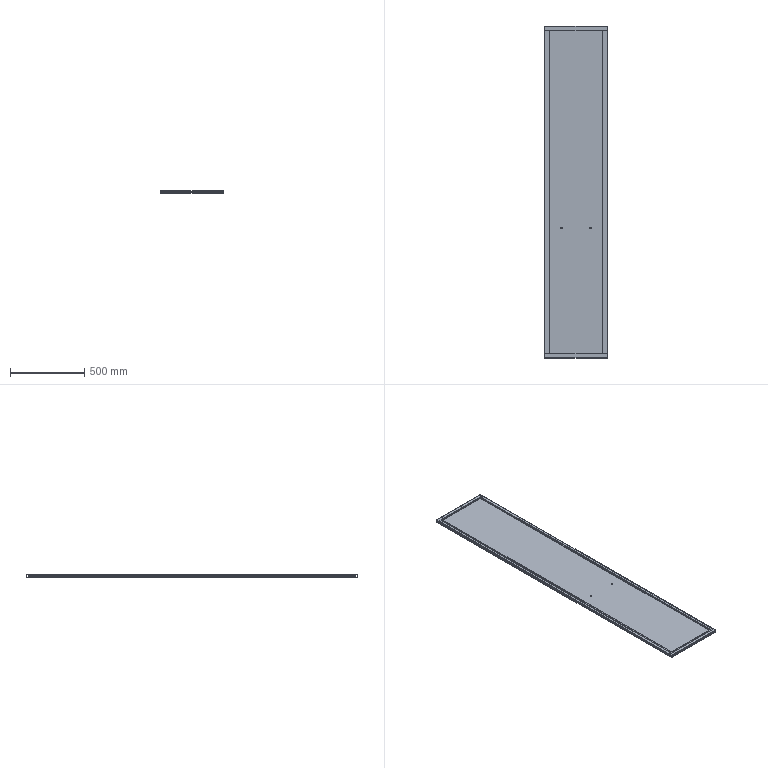Part | SolidWorks | features ICE 2, Cut 1, WeldMemberFeat 1, WeldmentFeature 1 | 5 solids | 171 faces | box 420 x 2236 x 18 mm | volume 9270830 mm3 | plane 98 | cylinder 73 | commonest cylinder face diameters 1.1 x24 3.6 x20 5.8 x20 1 x5 12 x4